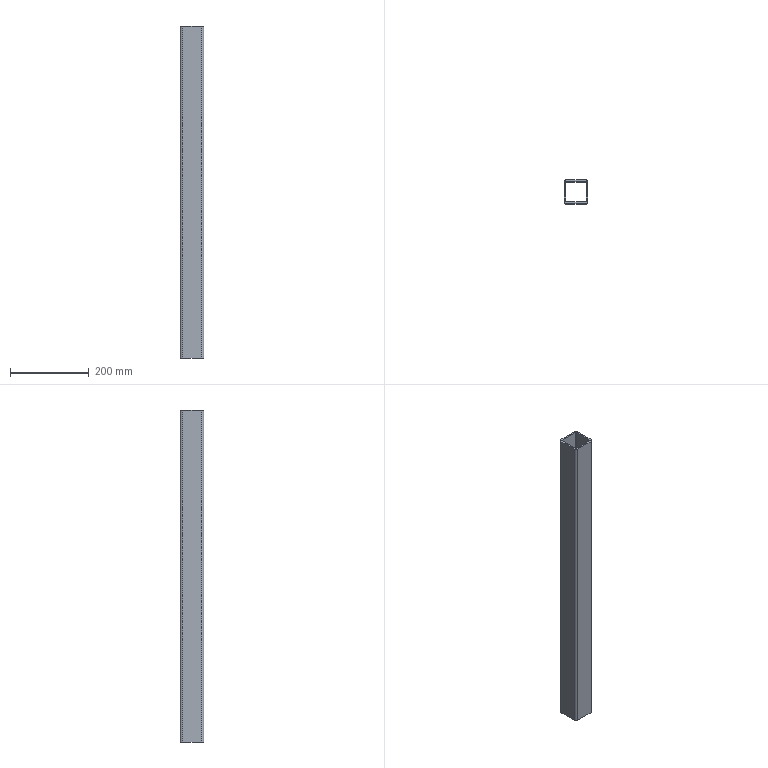Part | STEP file | 750038172 | 1 solid | 18 faces | box 60 x 60 x 841 mm | volume 730435 mm3 | plane 10 | cylinder 8 | commonest cylinder face diameters 4 x4 12 x4
STEP:
#1=CARTESIAN_POINT('',(-26.,24.,841.));
#2=VERTEX_POINT('',#1);
#3=CARTESIAN_POINT('',(-26.,24.,0.));
#4=VERTEX_POINT('',#3);
#5=CARTESIAN_POINT('',(-26.,24.,841.));
#6=DIRECTION('',(0.,0.,-1.));
#7=VECTOR('',#6,1000.);
#8=LINE('',#5,#7);
#9=EDGE_CURVE('',#2,#4,#8,.T.);
#10=ORIENTED_EDGE('',*,*,#9,.F.);
#11=CARTESIAN_POINT('',(-26.,-24.,841.));
#12=VERTEX_POINT('',#11);
#13=CARTESIAN_POINT('',(-26.,-24.,841.));
#14=DIRECTION('',(0.,1.,0.));
#15=VECTOR('',#14,1000.);
#16=LINE('',#13,#15);
#17=EDGE_CURVE('',#12,#2,#16,.T.);
#18=ORIENTED_EDGE('',*,*,#17,.F.);
#19=CARTESIAN_POINT('',(-26.,-24.,0.));
#20=VERTEX_POINT('',#19);
#21=CARTESIAN_POINT('',(-26.,-24.,841.));
#22=DIRECTION('',(0.,0.,1.));
#23=VECTOR('',#22,1000.);
#24=LINE('',#21,#23);
#25=EDGE_CURVE('',#20,#12,#24,.T.);
#26=ORIENTED_EDGE('',*,*,#25,.F.);
#27=CARTESIAN_POINT('',(-26.,-24.,0.));
#28=DIRECTION('',(0.,-1.,0.));
#29=VECTOR('',#28,1000.);
#30=LINE('',#27,#29);
#31=EDGE_CURVE('',#4,#20,#30,.T.);
#32=ORIENTED_EDGE('',*,*,#31,.F.);
#33=EDGE_LOOP('',(#10,#18,#26,#32));
#34=FACE_OUTER_BOUND('',#33,.T.);
#35=CARTESIAN_POINT('',(-26.,-24.,841.));
#36=DIRECTION('',(-1.,0.,0.));
#37=DIRECTION('',(0.,-1.,0.));
#38=AXIS2_PLACEMENT_3D('',#35,#36,#37);
#39=PLANE('',#38);
#40=ADVANCED_FACE('',(#34),#39,.F.);
#41=CARTESIAN_POINT('',(26.,24.,0.));
#42=VERTEX_POINT('',#41);
#43=CARTESIAN_POINT('',(24.,26.,0.));
#44=VERTEX_POINT('',#43);
#45=CARTESIAN_POINT('',(24.,24.,0.));
#46=DIRECTION('',(0.,0.,1.));
#47=DIRECTION('',(-1.,0.,0.));
#48=AXIS2_PLACEMENT_3D('',#45,#46,#47);
#49=CIRCLE('',#48,2.);
#50=EDGE_CURVE('',#42,#44,#49,.T.);
#51=ORIENTED_EDGE('',*,*,#50,.T.);
#52=CARTESIAN_POINT('',(-24.,26.,0.));
#53=VERTEX_POINT('',#52);
#54=CARTESIAN_POINT('',(24.,26.,0.));
#55=DIRECTION('',(-1.,0.,0.));
#56=VECTOR('',#55,1000.);
#57=LINE('',#54,#56);
#58=EDGE_CURVE('',#44,#53,#57,.T.);
#59=ORIENTED_EDGE('',*,*,#58,.T.);
#60=CARTESIAN_POINT('',(-24.,24.,0.));
#61=DIRECTION('',(0.,0.,1.));
#62=DIRECTION('',(-1.,0.,0.));
#63=AXIS2_PLACEMENT_3D('',#60,#61,#62);
#64=CIRCLE('',#63,2.);
#65=EDGE_CURVE('',#53,#4,#64,.T.);
#66=ORIENTED_EDGE('',*,*,#65,.T.);
#67=ORIENTED_EDGE('',*,*,#31,.T.);
#68=CARTESIAN_POINT('',(-24.,-26.,0.));
#69=VERTEX_POINT('',#68);
#70=CARTESIAN_POINT('',(-24.,-24.,0.));
#71=DIRECTION('',(0.,0.,1.));
#72=DIRECTION('',(-1.,0.,0.));
#73=AXIS2_PLACEMENT_3D('',#70,#71,#72);
#74=CIRCLE('',#73,2.);
#75=EDGE_CURVE('',#20,#69,#74,.T.);
#76=ORIENTED_EDGE('',*,*,#75,.T.);
#77=CARTESIAN_POINT('',(24.,-26.,0.));
#78=VERTEX_POINT('',#77);
#79=CARTESIAN_POINT('',(24.,-26.,0.));
#80=DIRECTION('',(1.,0.,0.));
#81=VECTOR('',#80,1000.);
#82=LINE('',#79,#81);
#83=EDGE_CURVE('',#69,#78,#82,.T.);
#84=ORIENTED_EDGE('',*,*,#83,.T.);
#85=CARTESIAN_POINT('',(26.,-24.,0.));
#86=VERTEX_POINT('',#85);
#87=CARTESIAN_POINT('',(24.,-24.,0.));
#88=DIRECTION('',(0.,0.,1.));
#89=DIRECTION('',(-1.,0.,0.));
#90=AXIS2_PLACEMENT_3D('',#87,#88,#89);
#91=CIRCLE('',#90,2.);
#92=EDGE_CURVE('',#78,#86,#91,.T.);
#93=ORIENTED_EDGE('',*,*,#92,.T.);
#94=CARTESIAN_POINT('',(26.,-24.,0.));
#95=DIRECTION('',(0.,1.,0.));
#96=VECTOR('',#95,1000.);
#97=LINE('',#94,#96);
#98=EDGE_CURVE('',#86,#42,#97,.T.);
#99=ORIENTED_EDGE('',*,*,#98,.T.);
#100=EDGE_LOOP('',(#51,#59,#66,#67,#76,#84,#93,#99));
#101=FACE_BOUND('',#100,.T.);
#102=CARTESIAN_POINT('',(-24.,30.,0.));
#103=VERTEX_POINT('',#102);
#104=CARTESIAN_POINT('',(24.,30.,0.));
#105=VERTEX_POINT('',#104);
#106=CARTESIAN_POINT('',(24.,30.,0.));
#107=DIRECTION('',(1.,0.,0.));
#108=VECTOR('',#107,1000.);
#109=LINE('',#106,#108);
#110=EDGE_CURVE('',#103,#105,#109,.T.);
#111=ORIENTED_EDGE('',*,*,#110,.T.);
#112=CARTESIAN_POINT('',(30.,24.,0.));
#113=VERTEX_POINT('',#112);
#114=CARTESIAN_POINT('',(24.,24.,0.));
#115=DIRECTION('',(0.,0.,-1.));
#116=DIRECTION('',(-1.,0.,0.));
#117=AXIS2_PLACEMENT_3D('',#114,#115,#116);
#118=CIRCLE('',#117,6.);
#119=EDGE_CURVE('',#105,#113,#118,.T.);
#120=ORIENTED_EDGE('',*,*,#119,.T.);
#121=CARTESIAN_POINT('',(30.,-24.,0.));
#122=VERTEX_POINT('',#121);
#123=CARTESIAN_POINT('',(30.,-24.,0.));
#124=DIRECTION('',(0.,-1.,0.));
#125=VECTOR('',#124,1000.);
#126=LINE('',#123,#125);
#127=EDGE_CURVE('',#113,#122,#126,.T.);
#128=ORIENTED_EDGE('',*,*,#127,.T.);
#129=CARTESIAN_POINT('',(24.,-30.,0.));
#130=VERTEX_POINT('',#129);
#131=CARTESIAN_POINT('',(24.,-24.,0.));
#132=DIRECTION('',(0.,0.,-1.));
#133=DIRECTION('',(-1.,0.,0.));
#134=AXIS2_PLACEMENT_3D('',#131,#132,#133);
#135=CIRCLE('',#134,6.);
#136=EDGE_CURVE('',#122,#130,#135,.T.);
#137=ORIENTED_EDGE('',*,*,#136,.T.);
#138=CARTESIAN_POINT('',(-24.,-30.,0.));
#139=VERTEX_POINT('',#138);
#140=CARTESIAN_POINT('',(24.,-30.,0.));
#141=DIRECTION('',(-1.,0.,0.));
#142=VECTOR('',#141,1000.);
#143=LINE('',#140,#142);
#144=EDGE_CURVE('',#130,#139,#143,.T.);
#145=ORIENTED_EDGE('',*,*,#144,.T.);
#146=CARTESIAN_POINT('',(-30.,-24.,0.));
#147=VERTEX_POINT('',#146);
#148=CARTESIAN_POINT('',(-24.,-24.,0.));
#149=DIRECTION('',(0.,0.,-1.));
#150=DIRECTION('',(-1.,0.,0.));
#151=AXIS2_PLACEMENT_3D('',#148,#149,#150);
#152=CIRCLE('',#151,6.);
#153=EDGE_CURVE('',#139,#147,#152,.T.);
#154=ORIENTED_EDGE('',*,*,#153,.T.);
#155=CARTESIAN_POINT('',(-30.,24.,0.));
#156=VERTEX_POINT('',#155);
#157=CARTESIAN_POINT('',(-30.,-24.,0.));
#158=DIRECTION('',(0.,1.,0.));
#159=VECTOR('',#158,1000.);
#160=LINE('',#157,#159);
#161=EDGE_CURVE('',#147,#156,#160,.T.);
#162=ORIENTED_EDGE('',*,*,#161,.T.);
#163=CARTESIAN_POINT('',(-24.,24.,0.));
#164=DIRECTION('',(0.,0.,-1.));
#165=DIRECTION('',(-1.,0.,0.));
#166=AXIS2_PLACEMENT_3D('',#163,#164,#165);
#167=CIRCLE('',#166,6.);
#168=EDGE_CURVE('',#156,#103,#167,.T.);
#169=ORIENTED_EDGE('',*,*,#168,.T.);
#170=EDGE_LOOP('',(#111,#120,#128,#137,#145,#154,#162,#169));
#171=FACE_OUTER_BOUND('',#170,.T.);
#172=CARTESIAN_POINT('',(24.,-24.,0.));
#173=DIRECTION('',(0.,0.,-1.));
#174=DIRECTION('',(-1.,0.,0.));
#175=AXIS2_PLACEMENT_3D('',#172,#173,#174);
#176=PLANE('',#175);
#177=ADVANCED_FACE('',(#101,#171),#176,.T.);
#178=CARTESIAN_POINT('',(-24.,26.,841.));
#179=VERTEX_POINT('',#178);
#180=CARTESIAN_POINT('',(-24.,26.,841.));
#181=DIRECTION('',(0.,0.,-1.));
#182=VECTOR('',#181,1000.);
#183=LINE('',#180,#182);
#184=EDGE_CURVE('',#179,#53,#183,.T.);
#185=ORIENTED_EDGE('',*,*,#184,.F.);
#186=CARTESIAN_POINT('',(-24.,24.,841.));
#187=DIRECTION('',(0.,0.,-1.));
#188=DIRECTION('',(-1.,0.,0.));
#189=AXIS2_PLACEMENT_3D('',#186,#187,#188);
#190=CIRCLE('',#189,2.);
#191=EDGE_CURVE('',#2,#179,#190,.T.);
#192=ORIENTED_EDGE('',*,*,#191,.F.);
#193=ORIENTED_EDGE('',*,*,#9,.T.);
#194=ORIENTED_EDGE('',*,*,#65,.F.);
#195=EDGE_LOOP('',(#185,#192,#193,#194));
#196=FACE_OUTER_BOUND('',#195,.T.);
#197=CARTESIAN_POINT('',(-24.,24.,841.));
#198=DIRECTION('',(0.,0.,-1.));
#199=DIRECTION('',(-1.,0.,0.));
#200=AXIS2_PLACEMENT_3D('',#197,#198,#199);
#201=CYLINDRICAL_SURFACE('',#200,2.);
#202=ADVANCED_FACE('',(#196),#201,.F.);
#203=CARTESIAN_POINT('',(24.,26.,841.));
#204=VERTEX_POINT('',#203);
#205=CARTESIAN_POINT('',(24.,26.,841.));
#206=DIRECTION('',(-1.,0.,0.));
#207=VECTOR('',#206,1000.);
#208=LINE('',#205,#207);
#209=EDGE_CURVE('',#204,#179,#208,.T.);
#210=ORIENTED_EDGE('',*,*,#209,.F.);
#211=CARTESIAN_POINT('',(26.,24.,841.));
#212=VERTEX_POINT('',#211);
#213=CARTESIAN_POINT('',(24.,24.,841.));
#214=DIRECTION('',(0.,0.,1.));
#215=DIRECTION('',(-1.,0.,0.));
#216=AXIS2_PLACEMENT_3D('',#213,#214,#215);
#217=CIRCLE('',#216,2.);
#218=EDGE_CURVE('',#212,#204,#217,.T.);
#219=ORIENTED_EDGE('',*,*,#218,.F.);
#220=CARTESIAN_POINT('',(26.,-24.,841.));
#221=VERTEX_POINT('',#220);
#222=CARTESIAN_POINT('',(26.,-24.,841.));
#223=DIRECTION('',(0.,1.,0.));
#224=VECTOR('',#223,1000.);
#225=LINE('',#222,#224);
#226=EDGE_CURVE('',#221,#212,#225,.T.);
#227=ORIENTED_EDGE('',*,*,#226,.F.);
#228=CARTESIAN_POINT('',(24.,-26.,841.));
#229=VERTEX_POINT('',#228);
#230=CARTESIAN_POINT('',(24.,-24.,841.));
#231=DIRECTION('',(0.,0.,1.));
#232=DIRECTION('',(-1.,0.,0.));
#233=AXIS2_PLACEMENT_3D('',#230,#231,#232);
#234=CIRCLE('',#233,2.);
#235=EDGE_CURVE('',#229,#221,#234,.T.);
#236=ORIENTED_EDGE('',*,*,#235,.F.);
#237=CARTESIAN_POINT('',(-24.,-26.,841.));
#238=VERTEX_POINT('',#237);
#239=CARTESIAN_POINT('',(24.,-26.,841.));
#240=DIRECTION('',(1.,0.,0.));
#241=VECTOR('',#240,1000.);
#242=LINE('',#239,#241);
#243=EDGE_CURVE('',#238,#229,#242,.T.);
#244=ORIENTED_EDGE('',*,*,#243,.F.);
#245=CARTESIAN_POINT('',(-24.,-24.,841.));
#246=DIRECTION('',(0.,0.,1.));
#247=DIRECTION('',(-1.,0.,0.));
#248=AXIS2_PLACEMENT_3D('',#245,#246,#247);
#249=CIRCLE('',#248,2.);
#250=EDGE_CURVE('',#12,#238,#249,.T.);
#251=ORIENTED_EDGE('',*,*,#250,.F.);
#252=ORIENTED_EDGE('',*,*,#17,.T.);
#253=ORIENTED_EDGE('',*,*,#191,.T.);
#254=EDGE_LOOP('',(#210,#219,#227,#236,#244,#251,#252,#253));
#255=FACE_BOUND('',#254,.T.);
#256=CARTESIAN_POINT('',(24.,30.,841.));
#257=VERTEX_POINT('',#256);
#258=CARTESIAN_POINT('',(30.,24.,841.));
#259=VERTEX_POINT('',#258);
#260=CARTESIAN_POINT('',(24.,24.,841.));
#261=DIRECTION('',(0.,0.,-1.));
#262=DIRECTION('',(-1.,0.,0.));
#263=AXIS2_PLACEMENT_3D('',#260,#261,#262);
#264=CIRCLE('',#263,6.);
#265=EDGE_CURVE('',#257,#259,#264,.T.);
#266=ORIENTED_EDGE('',*,*,#265,.F.);
#267=CARTESIAN_POINT('',(-24.,30.,841.));
#268=VERTEX_POINT('',#267);
#269=CARTESIAN_POINT('',(24.,30.,841.));
#270=DIRECTION('',(1.,0.,0.));
#271=VECTOR('',#270,1000.);
#272=LINE('',#269,#271);
#273=EDGE_CURVE('',#268,#257,#272,.T.);
#274=ORIENTED_EDGE('',*,*,#273,.F.);
#275=CARTESIAN_POINT('',(-30.,24.,841.));
#276=VERTEX_POINT('',#275);
#277=CARTESIAN_POINT('',(-24.,24.,841.));
#278=DIRECTION('',(0.,0.,-1.));
#279=DIRECTION('',(-1.,0.,0.));
#280=AXIS2_PLACEMENT_3D('',#277,#278,#279);
#281=CIRCLE('',#280,6.);
#282=EDGE_CURVE('',#276,#268,#281,.T.);
#283=ORIENTED_EDGE('',*,*,#282,.F.);
#284=CARTESIAN_POINT('',(-30.,-24.,841.));
#285=VERTEX_POINT('',#284);
#286=CARTESIAN_POINT('',(-30.,-24.,841.));
#287=DIRECTION('',(0.,1.,0.));
#288=VECTOR('',#287,1000.);
#289=LINE('',#286,#288);
#290=EDGE_CURVE('',#285,#276,#289,.T.);
#291=ORIENTED_EDGE('',*,*,#290,.F.);
#292=CARTESIAN_POINT('',(-24.,-30.,841.));
#293=VERTEX_POINT('',#292);
#294=CARTESIAN_POINT('',(-24.,-24.,841.));
#295=DIRECTION('',(0.,0.,-1.));
#296=DIRECTION('',(-1.,0.,0.));
#297=AXIS2_PLACEMENT_3D('',#294,#295,#296);
#298=CIRCLE('',#297,6.);
#299=EDGE_CURVE('',#293,#285,#298,.T.);
#300=ORIENTED_EDGE('',*,*,#299,.F.);
#301=CARTESIAN_POINT('',(24.,-30.,841.));
#302=VERTEX_POINT('',#301);
#303=CARTESIAN_POINT('',(24.,-30.,841.));
#304=DIRECTION('',(-1.,0.,0.));
#305=VECTOR('',#304,1000.);
#306=LINE('',#303,#305);
#307=EDGE_CURVE('',#302,#293,#306,.T.);
#308=ORIENTED_EDGE('',*,*,#307,.F.);
#309=CARTESIAN_POINT('',(30.,-24.,841.));
#310=VERTEX_POINT('',#309);
#311=CARTESIAN_POINT('',(24.,-24.,841.));
#312=DIRECTION('',(0.,0.,-1.));
#313=DIRECTION('',(-1.,0.,0.));
#314=AXIS2_PLACEMENT_3D('',#311,#312,#313);
#315=CIRCLE('',#314,6.);
#316=EDGE_CURVE('',#310,#302,#315,.T.);
#317=ORIENTED_EDGE('',*,*,#316,.F.);
#318=CARTESIAN_POINT('',(30.,-24.,841.));
#319=DIRECTION('',(0.,-1.,0.));
#320=VECTOR('',#319,1000.);
#321=LINE('',#318,#320);
#322=EDGE_CURVE('',#259,#310,#321,.T.);
#323=ORIENTED_EDGE('',*,*,#322,.F.);
#324=EDGE_LOOP('',(#266,#274,#283,#291,#300,#308,#317,#323));
#325=FACE_OUTER_BOUND('',#324,.T.);
#326=CARTESIAN_POINT('',(24.,-24.,841.));
#327=DIRECTION('',(0.,0.,-1.));
#328=DIRECTION('',(-1.,0.,0.));
#329=AXIS2_PLACEMENT_3D('',#326,#327,#328);
#330=PLANE('',#329);
#331=ADVANCED_FACE('',(#255,#325),#330,.F.);
#332=ORIENTED_EDGE('',*,*,#25,.T.);
#333=ORIENTED_EDGE('',*,*,#250,.T.);
#334=CARTESIAN_POINT('',(-24.,-26.,841.));
#335=DIRECTION('',(0.,0.,1.));
#336=VECTOR('',#335,1000.);
#337=LINE('',#334,#336);
#338=EDGE_CURVE('',#69,#238,#337,.T.);
#339=ORIENTED_EDGE('',*,*,#338,.F.);
#340=ORIENTED_EDGE('',*,*,#75,.F.);
#341=EDGE_LOOP('',(#332,#333,#339,#340));
#342=FACE_OUTER_BOUND('',#341,.T.);
#343=CARTESIAN_POINT('',(-24.,-24.,841.));
#344=DIRECTION('',(0.,0.,-1.));
#345=DIRECTION('',(-1.,0.,0.));
#346=AXIS2_PLACEMENT_3D('',#343,#344,#345);
#347=CYLINDRICAL_SURFACE('',#346,2.);
#348=ADVANCED_FACE('',(#342),#347,.F.);
#349=CARTESIAN_POINT('',(24.,26.,841.));
#350=DIRECTION('',(0.,0.,-1.));
#351=VECTOR('',#350,1000.);
#352=LINE('',#349,#351);
#353=EDGE_CURVE('',#204,#44,#352,.T.);
#354=ORIENTED_EDGE('',*,*,#353,.F.);
#355=ORIENTED_EDGE('',*,*,#209,.T.);
#356=ORIENTED_EDGE('',*,*,#184,.T.);
#357=ORIENTED_EDGE('',*,*,#58,.F.);
#358=EDGE_LOOP('',(#354,#355,#356,#357));
#359=FACE_OUTER_BOUND('',#358,.T.);
#360=CARTESIAN_POINT('',(-24.,26.,841.));
#361=DIRECTION('',(0.,1.,0.));
#362=DIRECTION('',(0.,0.,1.));
#363=AXIS2_PLACEMENT_3D('',#360,#361,#362);
#364=PLANE('',#363);
#365=ADVANCED_FACE('',(#359),#364,.F.);
#366=CARTESIAN_POINT('',(26.,24.,841.));
#367=DIRECTION('',(0.,0.,-1.));
#368=VECTOR('',#367,1000.);
#369=LINE('',#366,#368);
#370=EDGE_CURVE('',#212,#42,#369,.T.);
#371=ORIENTED_EDGE('',*,*,#370,.F.);
#372=ORIENTED_EDGE('',*,*,#218,.T.);
#373=ORIENTED_EDGE('',*,*,#353,.T.);
#374=ORIENTED_EDGE('',*,*,#50,.F.);
#375=EDGE_LOOP('',(#371,#372,#373,#374));
#376=FACE_OUTER_BOUND('',#375,.T.);
#377=CARTESIAN_POINT('',(24.,24.,841.));
#378=DIRECTION('',(0.,0.,-1.));
#379=DIRECTION('',(-1.,0.,0.));
#380=AXIS2_PLACEMENT_3D('',#377,#378,#379);
#381=CYLINDRICAL_SURFACE('',#380,2.);
#382=ADVANCED_FACE('',(#376),#381,.F.);
#383=CARTESIAN_POINT('',(26.,-24.,841.));
#384=DIRECTION('',(0.,0.,-1.));
#385=VECTOR('',#384,1000.);
#386=LINE('',#383,#385);
#387=EDGE_CURVE('',#221,#86,#386,.T.);
#388=ORIENTED_EDGE('',*,*,#387,.F.);
#389=ORIENTED_EDGE('',*,*,#226,.T.);
#390=ORIENTED_EDGE('',*,*,#370,.T.);
#391=ORIENTED_EDGE('',*,*,#98,.F.);
#392=EDGE_LOOP('',(#388,#389,#390,#391));
#393=FACE_OUTER_BOUND('',#392,.T.);
#394=CARTESIAN_POINT('',(26.,24.,841.));
#395=DIRECTION('',(1.,0.,0.));
#396=DIRECTION('',(0.,0.,-1.));
#397=AXIS2_PLACEMENT_3D('',#394,#395,#396);
#398=PLANE('',#397);
#399=ADVANCED_FACE('',(#393),#398,.F.);
#400=CARTESIAN_POINT('',(24.,-26.,841.));
#401=DIRECTION('',(0.,0.,-1.));
#402=VECTOR('',#401,1000.);
#403=LINE('',#400,#402);
#404=EDGE_CURVE('',#229,#78,#403,.T.);
#405=ORIENTED_EDGE('',*,*,#404,.F.);
#406=ORIENTED_EDGE('',*,*,#235,.T.);
#407=ORIENTED_EDGE('',*,*,#387,.T.);
#408=ORIENTED_EDGE('',*,*,#92,.F.);
#409=EDGE_LOOP('',(#405,#406,#407,#408));
#410=FACE_OUTER_BOUND('',#409,.T.);
#411=CARTESIAN_POINT('',(24.,-24.,841.));
#412=DIRECTION('',(0.,0.,-1.));
#413=DIRECTION('',(-1.,0.,0.));
#414=AXIS2_PLACEMENT_3D('',#411,#412,#413);
#415=CYLINDRICAL_SURFACE('',#414,2.);
#416=ADVANCED_FACE('',(#410),#415,.F.);
#417=ORIENTED_EDGE('',*,*,#338,.T.);
#418=ORIENTED_EDGE('',*,*,#243,.T.);
#419=ORIENTED_EDGE('',*,*,#404,.T.);
#420=ORIENTED_EDGE('',*,*,#83,.F.);
#421=EDGE_LOOP('',(#417,#418,#419,#420));
#422=FACE_OUTER_BOUND('',#421,.T.);
#423=CARTESIAN_POINT('',(24.,-26.,841.));
#424=DIRECTION('',(0.,-1.,0.));
#425=DIRECTION('',(0.,0.,-1.));
#426=AXIS2_PLACEMENT_3D('',#423,#424,#425);
#427=PLANE('',#426);
#428=ADVANCED_FACE('',(#422),#427,.F.);
#429=ORIENTED_EDGE('',*,*,#265,.T.);
#430=CARTESIAN_POINT('',(30.,24.,841.));
#431=DIRECTION('',(0.,0.,-1.));
#432=VECTOR('',#431,1000.);
#433=LINE('',#430,#432);
#434=EDGE_CURVE('',#259,#113,#433,.T.);
#435=ORIENTED_EDGE('',*,*,#434,.T.);
#436=ORIENTED_EDGE('',*,*,#119,.F.);
#437=CARTESIAN_POINT('',(24.,30.,841.));
#438=DIRECTION('',(0.,0.,1.));
#439=VECTOR('',#438,1000.);
#440=LINE('',#437,#439);
#441=EDGE_CURVE('',#105,#257,#440,.T.);
#442=ORIENTED_EDGE('',*,*,#441,.T.);
#443=EDGE_LOOP('',(#429,#435,#436,#442));
#444=FACE_OUTER_BOUND('',#443,.T.);
#445=CARTESIAN_POINT('',(24.,24.,841.));
#446=DIRECTION('',(0.,0.,-1.));
#447=DIRECTION('',(-1.,0.,0.));
#448=AXIS2_PLACEMENT_3D('',#445,#446,#447);
#449=CYLINDRICAL_SURFACE('',#448,6.);
#450=ADVANCED_FACE('',(#444),#449,.T.);
#451=ORIENTED_EDGE('',*,*,#273,.T.);
#452=ORIENTED_EDGE('',*,*,#441,.F.);
#453=ORIENTED_EDGE('',*,*,#110,.F.);
#454=CARTESIAN_POINT('',(-24.,30.,841.));
#455=DIRECTION('',(0.,0.,1.));
#456=VECTOR('',#455,1000.);
#457=LINE('',#454,#456);
#458=EDGE_CURVE('',#103,#268,#457,.T.);
#459=ORIENTED_EDGE('',*,*,#458,.T.);
#460=EDGE_LOOP('',(#451,#452,#453,#459));
#461=FACE_OUTER_BOUND('',#460,.T.);
#462=CARTESIAN_POINT('',(-24.,30.,841.));
#463=DIRECTION('',(0.,1.,0.));
#464=DIRECTION('',(-1.,0.,0.));
#465=AXIS2_PLACEMENT_3D('',#462,#463,#464);
#466=PLANE('',#465);
#467=ADVANCED_FACE('',(#461),#466,.T.);
#468=ORIENTED_EDGE('',*,*,#282,.T.);
#469=ORIENTED_EDGE('',*,*,#458,.F.);
#470=ORIENTED_EDGE('',*,*,#168,.F.);
#471=CARTESIAN_POINT('',(-30.,24.,841.));
#472=DIRECTION('',(0.,0.,1.));
#473=VECTOR('',#472,1000.);
#474=LINE('',#471,#473);
#475=EDGE_CURVE('',#156,#276,#474,.T.);
#476=ORIENTED_EDGE('',*,*,#475,.T.);
#477=EDGE_LOOP('',(#468,#469,#470,#476));
#478=FACE_OUTER_BOUND('',#477,.T.);
#479=CARTESIAN_POINT('',(-24.,24.,841.));
#480=DIRECTION('',(0.,0.,-1.));
#481=DIRECTION('',(-1.,0.,0.));
#482=AXIS2_PLACEMENT_3D('',#479,#480,#481);
#483=CYLINDRICAL_SURFACE('',#482,6.);
#484=ADVANCED_FACE('',(#478),#483,.T.);
#485=ORIENTED_EDGE('',*,*,#290,.T.);
#486=ORIENTED_EDGE('',*,*,#475,.F.);
#487=ORIENTED_EDGE('',*,*,#161,.F.);
#488=CARTESIAN_POINT('',(-30.,-24.,841.));
#489=DIRECTION('',(0.,0.,1.));
#490=VECTOR('',#489,1000.);
#491=LINE('',#488,#490);
#492=EDGE_CURVE('',#147,#285,#491,.T.);
#493=ORIENTED_EDGE('',*,*,#492,.T.);
#494=EDGE_LOOP('',(#485,#486,#487,#493));
#495=FACE_OUTER_BOUND('',#494,.T.);
#496=CARTESIAN_POINT('',(-30.,-24.,841.));
#497=DIRECTION('',(-1.,0.,0.));
#498=DIRECTION('',(0.,-1.,0.));
#499=AXIS2_PLACEMENT_3D('',#496,#497,#498);
#500=PLANE('',#499);
#501=ADVANCED_FACE('',(#495),#500,.T.);
#502=ORIENTED_EDGE('',*,*,#299,.T.);
#503=ORIENTED_EDGE('',*,*,#492,.F.);
#504=ORIENTED_EDGE('',*,*,#153,.F.);
#505=CARTESIAN_POINT('',(-24.,-30.,841.));
#506=DIRECTION('',(0.,0.,1.));
#507=VECTOR('',#506,1000.);
#508=LINE('',#505,#507);
#509=EDGE_CURVE('',#139,#293,#508,.T.);
#510=ORIENTED_EDGE('',*,*,#509,.T.);
#511=EDGE_LOOP('',(#502,#503,#504,#510));
#512=FACE_OUTER_BOUND('',#511,.T.);
#513=CARTESIAN_POINT('',(-24.,-24.,841.));
#514=DIRECTION('',(0.,0.,-1.));
#515=DIRECTION('',(-1.,0.,0.));
#516=AXIS2_PLACEMENT_3D('',#513,#514,#515);
#517=CYLINDRICAL_SURFACE('',#516,6.);
#518=ADVANCED_FACE('',(#512),#517,.T.);
#519=ORIENTED_EDGE('',*,*,#307,.T.);
#520=ORIENTED_EDGE('',*,*,#509,.F.);
#521=ORIENTED_EDGE('',*,*,#144,.F.);
#522=CARTESIAN_POINT('',(24.,-30.,841.));
#523=DIRECTION('',(0.,0.,1.));
#524=VECTOR('',#523,1000.);
#525=LINE('',#522,#524);
#526=EDGE_CURVE('',#130,#302,#525,.T.);
#527=ORIENTED_EDGE('',*,*,#526,.T.);
#528=EDGE_LOOP('',(#519,#520,#521,#527));
#529=FACE_OUTER_BOUND('',#528,.T.);
#530=CARTESIAN_POINT('',(24.,-30.,841.));
#531=DIRECTION('',(0.,-1.,0.));
#532=DIRECTION('',(1.,0.,0.));
#533=AXIS2_PLACEMENT_3D('',#530,#531,#532);
#534=PLANE('',#533);
#535=ADVANCED_FACE('',(#529),#534,.T.);
#536=ORIENTED_EDGE('',*,*,#316,.T.);
#537=ORIENTED_EDGE('',*,*,#526,.F.);
#538=ORIENTED_EDGE('',*,*,#136,.F.);
#539=CARTESIAN_POINT('',(30.,-24.,841.));
#540=DIRECTION('',(0.,0.,1.));
#541=VECTOR('',#540,1000.);
#542=LINE('',#539,#541);
#543=EDGE_CURVE('',#122,#310,#542,.T.);
#544=ORIENTED_EDGE('',*,*,#543,.T.);
#545=EDGE_LOOP('',(#536,#537,#538,#544));
#546=FACE_OUTER_BOUND('',#545,.T.);
#547=CARTESIAN_POINT('',(24.,-24.,841.));
#548=DIRECTION('',(0.,0.,-1.));
#549=DIRECTION('',(-1.,0.,0.));
#550=AXIS2_PLACEMENT_3D('',#547,#548,#549);
#551=CYLINDRICAL_SURFACE('',#550,6.);
#552=ADVANCED_FACE('',(#546),#551,.T.);
#553=ORIENTED_EDGE('',*,*,#322,.T.);
#554=ORIENTED_EDGE('',*,*,#543,.F.);
#555=ORIENTED_EDGE('',*,*,#127,.F.);
#556=ORIENTED_EDGE('',*,*,#434,.F.);
#557=EDGE_LOOP('',(#553,#554,#555,#556));
#558=FACE_OUTER_BOUND('',#557,.T.);
#559=CARTESIAN_POINT('',(30.,24.,841.));
#560=DIRECTION('',(1.,0.,0.));
#561=DIRECTION('',(0.,0.,-1.));
#562=AXIS2_PLACEMENT_3D('',#559,#560,#561);
#563=PLANE('',#562);
#564=ADVANCED_FACE('',(#558),#563,.T.);
#565=CLOSED_SHELL('',(#40,#177,#202,#331,#348,#365,#382,#399,#416,#428,#450,#467,#484,#501,#518,#535,#552,#564));
#566=MANIFOLD_SOLID_BREP('',#565);
#567=CARTESIAN_POINT('',(0.,0.,0.));
#568=DIRECTION('',(0.,0.,1.));
#569=DIRECTION('',(1.,0.,0.));
#570=AXIS2_PLACEMENT_3D('',#567,#568,#569);
#571=(LENGTH_UNIT()NAMED_UNIT(*)SI_UNIT(.MILLI.,.METRE.));
#572=UNCERTAINTY_MEASURE_WITH_UNIT(LENGTH_MEASURE(0.00001),#571,'','');
#573=(NAMED_UNIT(*)PLANE_ANGLE_UNIT()SI_UNIT($,.RADIAN.));
#574=(NAMED_UNIT(*)SI_UNIT($,.STERADIAN.)SOLID_ANGLE_UNIT());
#575=(GEOMETRIC_REPRESENTATION_CONTEXT(3)GLOBAL_UNCERTAINTY_ASSIGNED_CONTEXT((#572))GLOBAL_UNIT_ASSIGNED_CONTEXT((#571,#573,#574))REPRESENTATION_CONTEXT('',''));
#576=ADVANCED_BREP_SHAPE_REPRESENTATION('',(#566,#570),#575);